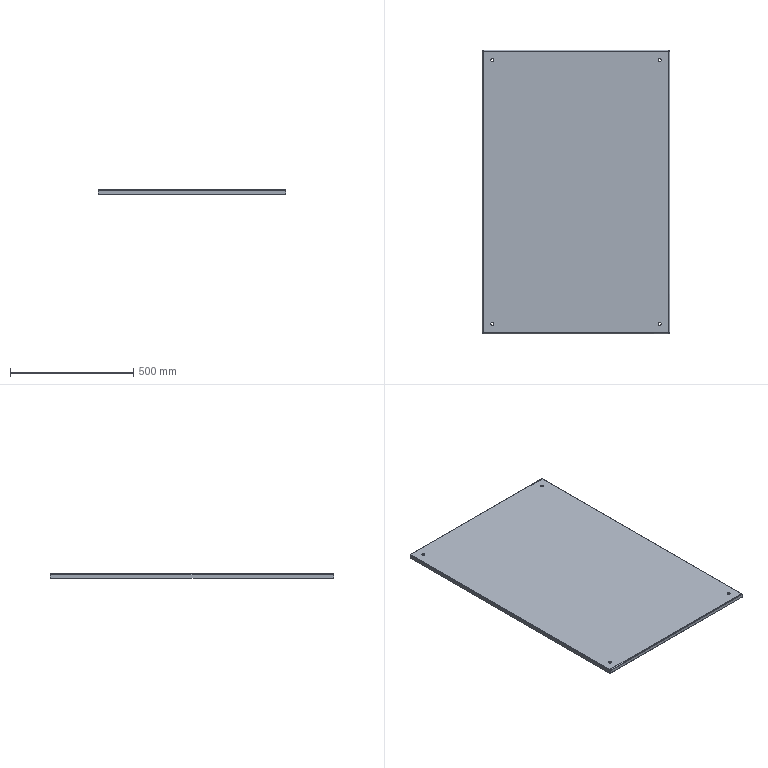Part | NX | features BREP 1 | 1 solid | 46 faces | box 760 x 1150 x 17 mm | volume 1851169 mm3 | plane 22 | cylinder 16 | spline 8 | commonest cylinder face diameters 12 x8 4 x4 8 x4